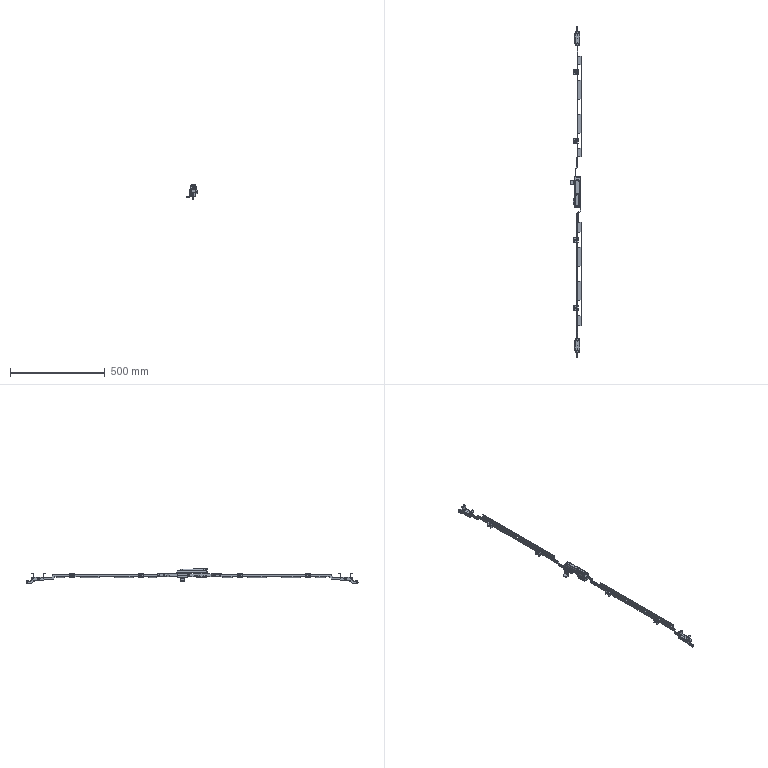Part | SolidWorks | 15 solids | 3848 faces | volume 354864 mm3 | plane 2013 | cylinder 1179 | spline 567 | cone 74 | torus 15 | commonest cylinder face diameters 1 x235 4.1 x102 2 x89 4.8 x86 3 x63 0.2 x61